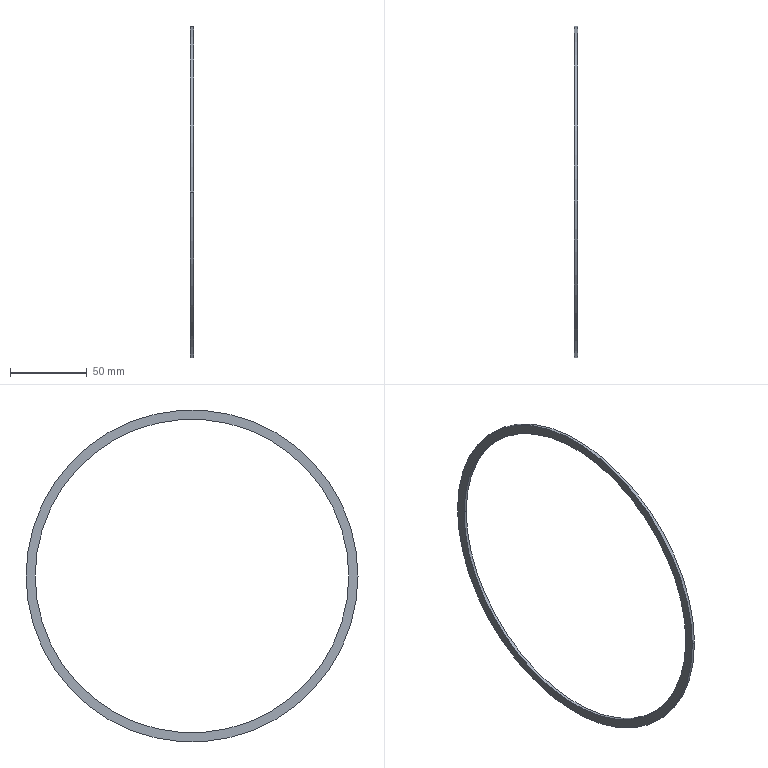Part | NX | features BREP 1 | 1 solid | 6 faces | box 2 x 216 x 216 mm | volume 7917 mm3 | cylinder 4 | plane 2 | commonest cylinder face diameters 204 x2 216 x2
STEP:
#1=CARTESIAN_POINT('',(-452.355,102.,0.));
#2=VERTEX_POINT('',#1);
#3=CARTESIAN_POINT('',(-452.355,-102.,0.));
#4=VERTEX_POINT('',#3);
#5=CARTESIAN_POINT('',(-452.355,0.,0.));
#6=DIRECTION('',(1.,0.,0.));
#7=DIRECTION('',(0.,-1.,0.));
#8=AXIS2_PLACEMENT_3D('',#5,#6,#7);
#9=CIRCLE('',#8,102.);
#10=EDGE_CURVE('',#2,#4,#9,.T.);
#11=ORIENTED_EDGE('',*,*,#10,.T.);
#12=CARTESIAN_POINT('',(-454.355,-102.,0.));
#13=VERTEX_POINT('',#12);
#14=CARTESIAN_POINT('',(-452.355,-102.,0.));
#15=DIRECTION('',(-1.,0.,0.));
#16=VECTOR('',#15,1000.);
#17=LINE('',#14,#16);
#18=EDGE_CURVE('',#4,#13,#17,.T.);
#19=ORIENTED_EDGE('',*,*,#18,.T.);
#20=CARTESIAN_POINT('',(-454.355,102.,0.));
#21=VERTEX_POINT('',#20);
#22=CARTESIAN_POINT('',(-454.355,0.,0.));
#23=DIRECTION('',(1.,0.,0.));
#24=DIRECTION('',(0.,-1.,0.));
#25=AXIS2_PLACEMENT_3D('',#22,#23,#24);
#26=CIRCLE('',#25,102.);
#27=EDGE_CURVE('',#21,#13,#26,.T.);
#28=ORIENTED_EDGE('',*,*,#27,.F.);
#29=CARTESIAN_POINT('',(-452.355,102.,0.));
#30=DIRECTION('',(-1.,0.,0.));
#31=VECTOR('',#30,1000.);
#32=LINE('',#29,#31);
#33=EDGE_CURVE('',#2,#21,#32,.T.);
#34=ORIENTED_EDGE('',*,*,#33,.F.);
#35=EDGE_LOOP('',(#11,#19,#28,#34));
#36=FACE_BOUND('',#35,.T.);
#37=CARTESIAN_POINT('',(-452.355,0.,0.));
#38=DIRECTION('',(-1.,0.,0.));
#39=DIRECTION('',(0.,1.,0.));
#40=AXIS2_PLACEMENT_3D('',#37,#38,#39);
#41=CYLINDRICAL_SURFACE('',#40,102.);
#42=ADVANCED_FACE('',(#36),#41,.F.);
#43=CARTESIAN_POINT('',(-452.355,-108.,0.));
#44=VERTEX_POINT('',#43);
#45=CARTESIAN_POINT('',(-452.355,108.,0.));
#46=VERTEX_POINT('',#45);
#47=CARTESIAN_POINT('',(-452.355,0.,0.));
#48=DIRECTION('',(1.,0.,0.));
#49=DIRECTION('',(0.,-1.,0.));
#50=AXIS2_PLACEMENT_3D('',#47,#48,#49);
#51=CIRCLE('',#50,108.);
#52=EDGE_CURVE('',#44,#46,#51,.T.);
#53=ORIENTED_EDGE('',*,*,#52,.F.);
#54=CARTESIAN_POINT('',(-454.355,-108.,0.));
#55=VERTEX_POINT('',#54);
#56=CARTESIAN_POINT('',(-452.355,-108.,0.));
#57=DIRECTION('',(-1.,0.,0.));
#58=VECTOR('',#57,1000.);
#59=LINE('',#56,#58);
#60=EDGE_CURVE('',#44,#55,#59,.T.);
#61=ORIENTED_EDGE('',*,*,#60,.T.);
#62=CARTESIAN_POINT('',(-454.355,108.,0.));
#63=VERTEX_POINT('',#62);
#64=CARTESIAN_POINT('',(-454.355,0.,0.));
#65=DIRECTION('',(1.,0.,0.));
#66=DIRECTION('',(0.,-1.,0.));
#67=AXIS2_PLACEMENT_3D('',#64,#65,#66);
#68=CIRCLE('',#67,108.);
#69=EDGE_CURVE('',#55,#63,#68,.T.);
#70=ORIENTED_EDGE('',*,*,#69,.T.);
#71=CARTESIAN_POINT('',(-452.355,108.,0.));
#72=DIRECTION('',(-1.,0.,0.));
#73=VECTOR('',#72,1000.);
#74=LINE('',#71,#73);
#75=EDGE_CURVE('',#46,#63,#74,.T.);
#76=ORIENTED_EDGE('',*,*,#75,.F.);
#77=EDGE_LOOP('',(#53,#61,#70,#76));
#78=FACE_BOUND('',#77,.T.);
#79=CARTESIAN_POINT('',(-452.355,0.,0.));
#80=DIRECTION('',(-1.,0.,0.));
#81=DIRECTION('',(0.,1.,0.));
#82=AXIS2_PLACEMENT_3D('',#79,#80,#81);
#83=CYLINDRICAL_SURFACE('',#82,108.);
#84=ADVANCED_FACE('',(#78),#83,.T.);
#85=CARTESIAN_POINT('',(-452.355,0.,0.));
#86=DIRECTION('',(1.,0.,0.));
#87=DIRECTION('',(0.,-1.,0.));
#88=AXIS2_PLACEMENT_3D('',#85,#86,#87);
#89=CIRCLE('',#88,108.);
#90=EDGE_CURVE('',#46,#44,#89,.T.);
#91=ORIENTED_EDGE('',*,*,#90,.T.);
#92=ORIENTED_EDGE('',*,*,#52,.T.);
#93=EDGE_LOOP('',(#91,#92));
#94=FACE_BOUND('',#93,.T.);
#95=ORIENTED_EDGE('',*,*,#10,.F.);
#96=CARTESIAN_POINT('',(-452.355,0.,0.));
#97=DIRECTION('',(1.,0.,0.));
#98=DIRECTION('',(0.,-1.,0.));
#99=AXIS2_PLACEMENT_3D('',#96,#97,#98);
#100=CIRCLE('',#99,102.);
#101=EDGE_CURVE('',#4,#2,#100,.T.);
#102=ORIENTED_EDGE('',*,*,#101,.F.);
#103=EDGE_LOOP('',(#95,#102));
#104=FACE_BOUND('',#103,.T.);
#105=CARTESIAN_POINT('',(-452.355,0.,0.));
#106=DIRECTION('',(1.,0.,0.));
#107=DIRECTION('',(0.,-1.,0.));
#108=AXIS2_PLACEMENT_3D('',#105,#106,#107);
#109=PLANE('',#108);
#110=ADVANCED_FACE('',(#94,#104),#109,.T.);
#111=CARTESIAN_POINT('',(-454.355,0.,0.));
#112=DIRECTION('',(1.,0.,0.));
#113=DIRECTION('',(0.,-1.,0.));
#114=AXIS2_PLACEMENT_3D('',#111,#112,#113);
#115=CIRCLE('',#114,108.);
#116=EDGE_CURVE('',#63,#55,#115,.T.);
#117=ORIENTED_EDGE('',*,*,#116,.F.);
#118=ORIENTED_EDGE('',*,*,#69,.F.);
#119=EDGE_LOOP('',(#117,#118));
#120=FACE_BOUND('',#119,.T.);
#121=ORIENTED_EDGE('',*,*,#27,.T.);
#122=CARTESIAN_POINT('',(-454.355,0.,0.));
#123=DIRECTION('',(1.,0.,0.));
#124=DIRECTION('',(0.,-1.,0.));
#125=AXIS2_PLACEMENT_3D('',#122,#123,#124);
#126=CIRCLE('',#125,102.);
#127=EDGE_CURVE('',#13,#21,#126,.T.);
#128=ORIENTED_EDGE('',*,*,#127,.T.);
#129=EDGE_LOOP('',(#121,#128));
#130=FACE_BOUND('',#129,.T.);
#131=CARTESIAN_POINT('',(-454.355,0.,0.));
#132=DIRECTION('',(1.,0.,0.));
#133=DIRECTION('',(0.,-1.,0.));
#134=AXIS2_PLACEMENT_3D('',#131,#132,#133);
#135=PLANE('',#134);
#136=ADVANCED_FACE('',(#120,#130),#135,.F.);
#137=ORIENTED_EDGE('',*,*,#60,.F.);
#138=ORIENTED_EDGE('',*,*,#90,.F.);
#139=ORIENTED_EDGE('',*,*,#75,.T.);
#140=ORIENTED_EDGE('',*,*,#116,.T.);
#141=EDGE_LOOP('',(#137,#138,#139,#140));
#142=FACE_BOUND('',#141,.T.);
#143=CARTESIAN_POINT('',(-452.355,0.,0.));
#144=DIRECTION('',(-1.,0.,0.));
#145=DIRECTION('',(0.,1.,0.));
#146=AXIS2_PLACEMENT_3D('',#143,#144,#145);
#147=CYLINDRICAL_SURFACE('',#146,108.);
#148=ADVANCED_FACE('',(#142),#147,.T.);
#149=ORIENTED_EDGE('',*,*,#18,.F.);
#150=ORIENTED_EDGE('',*,*,#101,.T.);
#151=ORIENTED_EDGE('',*,*,#33,.T.);
#152=ORIENTED_EDGE('',*,*,#127,.F.);
#153=EDGE_LOOP('',(#149,#150,#151,#152));
#154=FACE_BOUND('',#153,.T.);
#155=CARTESIAN_POINT('',(-452.355,0.,0.));
#156=DIRECTION('',(-1.,0.,0.));
#157=DIRECTION('',(0.,1.,0.));
#158=AXIS2_PLACEMENT_3D('',#155,#156,#157);
#159=CYLINDRICAL_SURFACE('',#158,102.);
#160=ADVANCED_FACE('',(#154),#159,.F.);
#161=CLOSED_SHELL('',(#42,#84,#110,#136,#148,#160));
#162=MANIFOLD_SOLID_BREP('',#161);
#163=(LENGTH_UNIT()NAMED_UNIT(*)SI_UNIT(.MILLI.,.METRE.));
#164=UNCERTAINTY_MEASURE_WITH_UNIT(LENGTH_MEASURE(0.00001),#163,'','');
#165=(NAMED_UNIT(*)PLANE_ANGLE_UNIT()SI_UNIT($,.RADIAN.));
#166=(NAMED_UNIT(*)SI_UNIT($,.STERADIAN.)SOLID_ANGLE_UNIT());
#167=(GEOMETRIC_REPRESENTATION_CONTEXT(3)GLOBAL_UNCERTAINTY_ASSIGNED_CONTEXT((#164))GLOBAL_UNIT_ASSIGNED_CONTEXT((#163,#165,#166))REPRESENTATION_CONTEXT('',''));
#168=ADVANCED_BREP_SHAPE_REPRESENTATION('',(#162),#167);